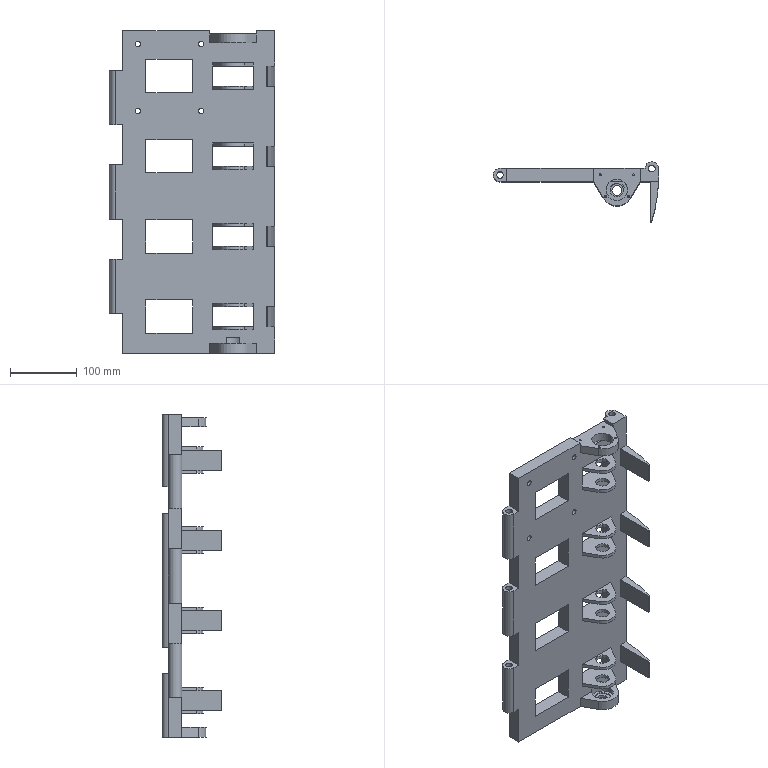Part | SolidWorks | features BaseBody 1 | 1 solid | 197 faces | box 247.548 x 89.579 x 483 mm | volume 1972744 mm3 | plane 118 | cylinder 79 | commonest cylinder face diameters 20 x32 10 x12 3 x8 8 x8 40 x8 32 x4